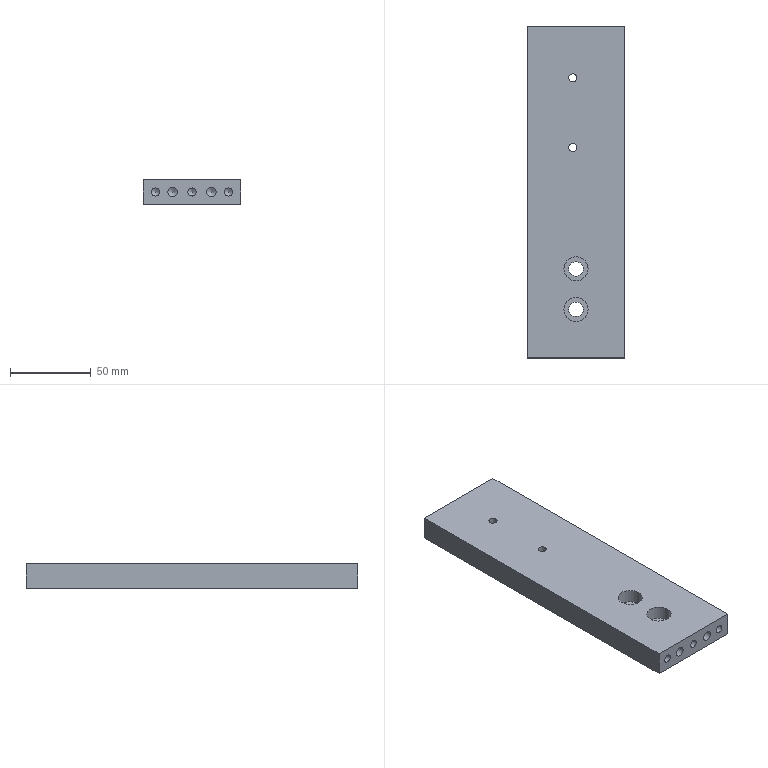Part | NX | features BREP 1 | 1 solid | 28 faces | box 60 x 205 x 15 mm | volume 177777 mm3 | cylinder 13 | plane 10 | cone 5 | commonest cylinder face diameters 5 x5 6 x2 9 x2 12 x2 15 x2
STEP:
#1=CARTESIAN_POINT('',(-4.5,27.5,7.5));
#2=VERTEX_POINT('',#1);
#3=CARTESIAN_POINT('',(-2.,27.5,7.5));
#4=DIRECTION('',(0.,0.,-1.));
#5=DIRECTION('',(-1.,0.,0.));
#6=AXIS2_PLACEMENT_3D('',#3,#4,#5);
#7=CIRCLE('',#6,2.5);
#8=EDGE_CURVE('',#2,#2,#7,.T.);
#9=ORIENTED_EDGE('',*,*,#8,.F.);
#10=EDGE_LOOP('',(#9));
#11=FACE_BOUND('',#10,.T.);
#12=CARTESIAN_POINT('',(-4.5,27.5,-4.));
#13=VERTEX_POINT('',#12);
#14=CARTESIAN_POINT('',(-2.,27.5,-4.));
#15=DIRECTION('',(0.,0.,1.));
#16=DIRECTION('',(-1.,0.,0.));
#17=AXIS2_PLACEMENT_3D('',#14,#15,#16);
#18=CIRCLE('',#17,2.5);
#19=EDGE_CURVE('',#13,#13,#18,.T.);
#20=ORIENTED_EDGE('',*,*,#19,.F.);
#21=EDGE_LOOP('',(#20));
#22=FACE_BOUND('',#21,.T.);
#23=CARTESIAN_POINT('',(-2.,27.5,-7.5));
#24=DIRECTION('',(0.,0.,-1.));
#25=DIRECTION('',(1.,0.,0.));
#26=AXIS2_PLACEMENT_3D('',#23,#24,#25);
#27=CYLINDRICAL_SURFACE('',#26,2.5);
#28=ADVANCED_FACE('',(#11,#22),#27,.F.);
#29=CARTESIAN_POINT('',(-4.5,70.5,7.5));
#30=VERTEX_POINT('',#29);
#31=CARTESIAN_POINT('',(-2.,70.5,7.5));
#32=DIRECTION('',(0.,0.,-1.));
#33=DIRECTION('',(-1.,0.,0.));
#34=AXIS2_PLACEMENT_3D('',#31,#32,#33);
#35=CIRCLE('',#34,2.5);
#36=EDGE_CURVE('',#30,#30,#35,.T.);
#37=ORIENTED_EDGE('',*,*,#36,.F.);
#38=EDGE_LOOP('',(#37));
#39=FACE_BOUND('',#38,.T.);
#40=CARTESIAN_POINT('',(-4.5,70.5,-4.));
#41=VERTEX_POINT('',#40);
#42=CARTESIAN_POINT('',(-2.,70.5,-4.));
#43=DIRECTION('',(0.,0.,1.));
#44=DIRECTION('',(-1.,0.,0.));
#45=AXIS2_PLACEMENT_3D('',#42,#43,#44);
#46=CIRCLE('',#45,2.5);
#47=EDGE_CURVE('',#41,#41,#46,.T.);
#48=ORIENTED_EDGE('',*,*,#47,.F.);
#49=EDGE_LOOP('',(#48));
#50=FACE_BOUND('',#49,.T.);
#51=CARTESIAN_POINT('',(-2.,70.5,-7.5));
#52=DIRECTION('',(0.,0.,-1.));
#53=DIRECTION('',(1.,0.,0.));
#54=AXIS2_PLACEMENT_3D('',#51,#52,#53);
#55=CYLINDRICAL_SURFACE('',#54,2.5);
#56=ADVANCED_FACE('',(#39,#50),#55,.F.);
#57=CARTESIAN_POINT('',(30.,-102.5,-7.5));
#58=VERTEX_POINT('',#57);
#59=CARTESIAN_POINT('',(30.,102.5,-7.5));
#60=VERTEX_POINT('',#59);
#61=CARTESIAN_POINT('',(30.,-102.5,-7.5));
#62=DIRECTION('',(0.,1.,0.));
#63=VECTOR('',#62,1000.);
#64=LINE('',#61,#63);
#65=EDGE_CURVE('',#58,#60,#64,.T.);
#66=ORIENTED_EDGE('',*,*,#65,.T.);
#67=CARTESIAN_POINT('',(30.,102.5,7.5));
#68=VERTEX_POINT('',#67);
#69=CARTESIAN_POINT('',(30.,102.5,7.5));
#70=DIRECTION('',(0.,0.,-1.));
#71=VECTOR('',#70,1000.);
#72=LINE('',#69,#71);
#73=EDGE_CURVE('',#68,#60,#72,.T.);
#74=ORIENTED_EDGE('',*,*,#73,.F.);
#75=CARTESIAN_POINT('',(30.,-102.5,7.5));
#76=VERTEX_POINT('',#75);
#77=CARTESIAN_POINT('',(30.,-102.5,7.5));
#78=DIRECTION('',(0.,1.,0.));
#79=VECTOR('',#78,1000.);
#80=LINE('',#77,#79);
#81=EDGE_CURVE('',#76,#68,#80,.T.);
#82=ORIENTED_EDGE('',*,*,#81,.F.);
#83=CARTESIAN_POINT('',(30.,-102.5,7.5));
#84=DIRECTION('',(0.,0.,-1.));
#85=VECTOR('',#84,1000.);
#86=LINE('',#83,#85);
#87=EDGE_CURVE('',#76,#58,#86,.T.);
#88=ORIENTED_EDGE('',*,*,#87,.T.);
#89=EDGE_LOOP('',(#66,#74,#82,#88));
#90=FACE_BOUND('',#89,.T.);
#91=CARTESIAN_POINT('',(30.,-102.5,7.5));
#92=DIRECTION('',(-1.,0.,0.));
#93=DIRECTION('',(0.,0.,-1.));
#94=AXIS2_PLACEMENT_3D('',#91,#92,#93);
#95=PLANE('',#94);
#96=ADVANCED_FACE('',(#90),#95,.F.);
#97=CARTESIAN_POINT('',(-30.,102.5,-7.5));
#98=VERTEX_POINT('',#97);
#99=CARTESIAN_POINT('',(-30.,102.5,-7.5));
#100=DIRECTION('',(-1.,0.,0.));
#101=VECTOR('',#100,1000.);
#102=LINE('',#99,#101);
#103=EDGE_CURVE('',#60,#98,#102,.T.);
#104=ORIENTED_EDGE('',*,*,#103,.T.);
#105=CARTESIAN_POINT('',(-30.,102.5,7.5));
#106=VERTEX_POINT('',#105);
#107=CARTESIAN_POINT('',(-30.,102.5,7.5));
#108=DIRECTION('',(0.,0.,-1.));
#109=VECTOR('',#108,1000.);
#110=LINE('',#107,#109);
#111=EDGE_CURVE('',#106,#98,#110,.T.);
#112=ORIENTED_EDGE('',*,*,#111,.F.);
#113=CARTESIAN_POINT('',(-30.,102.5,7.5));
#114=DIRECTION('',(-1.,0.,0.));
#115=VECTOR('',#114,1000.);
#116=LINE('',#113,#115);
#117=EDGE_CURVE('',#68,#106,#116,.T.);
#118=ORIENTED_EDGE('',*,*,#117,.F.);
#119=ORIENTED_EDGE('',*,*,#73,.T.);
#120=EDGE_LOOP('',(#104,#112,#118,#119));
#121=FACE_BOUND('',#120,.T.);
#122=CARTESIAN_POINT('',(-30.,102.5,7.5));
#123=DIRECTION('',(0.,-1.,0.));
#124=DIRECTION('',(0.,0.,1.));
#125=AXIS2_PLACEMENT_3D('',#122,#123,#124);
#126=PLANE('',#125);
#127=ADVANCED_FACE('',(#121),#126,.F.);
#128=CARTESIAN_POINT('',(-30.,-102.5,-7.5));
#129=VERTEX_POINT('',#128);
#130=CARTESIAN_POINT('',(-30.,-102.5,-7.5));
#131=DIRECTION('',(0.,-1.,0.));
#132=VECTOR('',#131,1000.);
#133=LINE('',#130,#132);
#134=EDGE_CURVE('',#98,#129,#133,.T.);
#135=ORIENTED_EDGE('',*,*,#134,.T.);
#136=CARTESIAN_POINT('',(-30.,-102.5,7.5));
#137=VERTEX_POINT('',#136);
#138=CARTESIAN_POINT('',(-30.,-102.5,7.5));
#139=DIRECTION('',(0.,0.,-1.));
#140=VECTOR('',#139,1000.);
#141=LINE('',#138,#140);
#142=EDGE_CURVE('',#137,#129,#141,.T.);
#143=ORIENTED_EDGE('',*,*,#142,.F.);
#144=CARTESIAN_POINT('',(-30.,-102.5,7.5));
#145=DIRECTION('',(0.,-1.,0.));
#146=VECTOR('',#145,1000.);
#147=LINE('',#144,#146);
#148=EDGE_CURVE('',#106,#137,#147,.T.);
#149=ORIENTED_EDGE('',*,*,#148,.F.);
#150=ORIENTED_EDGE('',*,*,#111,.T.);
#151=EDGE_LOOP('',(#135,#143,#149,#150));
#152=FACE_BOUND('',#151,.T.);
#153=CARTESIAN_POINT('',(-30.,-102.5,7.5));
#154=DIRECTION('',(1.,0.,0.));
#155=DIRECTION('',(0.,0.,1.));
#156=AXIS2_PLACEMENT_3D('',#153,#154,#155);
#157=PLANE('',#156);
#158=ADVANCED_FACE('',(#152),#157,.F.);
#159=CARTESIAN_POINT('',(-22.5,-102.5,-2.5));
#160=VERTEX_POINT('',#159);
#161=CARTESIAN_POINT('',(-22.5,-102.5,0.));
#162=DIRECTION('',(0.,-1.,0.));
#163=DIRECTION('',(0.,0.,-1.));
#164=AXIS2_PLACEMENT_3D('',#161,#162,#163);
#165=CIRCLE('',#164,2.5);
#166=EDGE_CURVE('',#160,#160,#165,.T.);
#167=ORIENTED_EDGE('',*,*,#166,.F.);
#168=EDGE_LOOP('',(#167));
#169=FACE_BOUND('',#168,.T.);
#170=CARTESIAN_POINT('',(0.,-102.5,-2.5));
#171=VERTEX_POINT('',#170);
#172=CARTESIAN_POINT('',(0.,-102.5,0.));
#173=DIRECTION('',(0.,-1.,0.));
#174=DIRECTION('',(0.,0.,-1.));
#175=AXIS2_PLACEMENT_3D('',#172,#173,#174);
#176=CIRCLE('',#175,2.5);
#177=EDGE_CURVE('',#171,#171,#176,.T.);
#178=ORIENTED_EDGE('',*,*,#177,.F.);
#179=EDGE_LOOP('',(#178));
#180=FACE_BOUND('',#179,.T.);
#181=CARTESIAN_POINT('',(22.5,-102.5,-2.5));
#182=VERTEX_POINT('',#181);
#183=CARTESIAN_POINT('',(22.5,-102.5,0.));
#184=DIRECTION('',(0.,-1.,0.));
#185=DIRECTION('',(0.,0.,-1.));
#186=AXIS2_PLACEMENT_3D('',#183,#184,#185);
#187=CIRCLE('',#186,2.5);
#188=EDGE_CURVE('',#182,#182,#187,.T.);
#189=ORIENTED_EDGE('',*,*,#188,.F.);
#190=EDGE_LOOP('',(#189));
#191=FACE_BOUND('',#190,.T.);
#192=CARTESIAN_POINT('',(12.,-102.5,-3.));
#193=VERTEX_POINT('',#192);
#194=CARTESIAN_POINT('',(12.,-102.5,0.));
#195=DIRECTION('',(0.,-1.,0.));
#196=DIRECTION('',(0.,0.,-1.));
#197=AXIS2_PLACEMENT_3D('',#194,#195,#196);
#198=CIRCLE('',#197,3.);
#199=EDGE_CURVE('',#193,#193,#198,.T.);
#200=ORIENTED_EDGE('',*,*,#199,.F.);
#201=EDGE_LOOP('',(#200));
#202=FACE_BOUND('',#201,.T.);
#203=CARTESIAN_POINT('',(-12.,-102.5,-3.));
#204=VERTEX_POINT('',#203);
#205=CARTESIAN_POINT('',(-12.,-102.5,0.));
#206=DIRECTION('',(0.,-1.,0.));
#207=DIRECTION('',(0.,0.,-1.));
#208=AXIS2_PLACEMENT_3D('',#205,#206,#207);
#209=CIRCLE('',#208,3.);
#210=EDGE_CURVE('',#204,#204,#209,.T.);
#211=ORIENTED_EDGE('',*,*,#210,.F.);
#212=EDGE_LOOP('',(#211));
#213=FACE_BOUND('',#212,.T.);
#214=CARTESIAN_POINT('',(-30.,-102.5,-7.5));
#215=DIRECTION('',(1.,0.,0.));
#216=VECTOR('',#215,1000.);
#217=LINE('',#214,#216);
#218=EDGE_CURVE('',#129,#58,#217,.T.);
#219=ORIENTED_EDGE('',*,*,#218,.T.);
#220=ORIENTED_EDGE('',*,*,#87,.F.);
#221=CARTESIAN_POINT('',(-30.,-102.5,7.5));
#222=DIRECTION('',(1.,0.,0.));
#223=VECTOR('',#222,1000.);
#224=LINE('',#221,#223);
#225=EDGE_CURVE('',#137,#76,#224,.T.);
#226=ORIENTED_EDGE('',*,*,#225,.F.);
#227=ORIENTED_EDGE('',*,*,#142,.T.);
#228=EDGE_LOOP('',(#219,#220,#226,#227));
#229=FACE_BOUND('',#228,.T.);
#230=CARTESIAN_POINT('',(-30.,-102.5,7.5));
#231=DIRECTION('',(0.,1.,0.));
#232=DIRECTION('',(0.,0.,-1.));
#233=AXIS2_PLACEMENT_3D('',#230,#231,#232);
#234=PLANE('',#233);
#235=ADVANCED_FACE('',(#169,#180,#191,#202,#213,#229),#234,.F.);
#236=CARTESIAN_POINT('',(7.5,-72.5,7.5));
#237=VERTEX_POINT('',#236);
#238=CARTESIAN_POINT('',(0.,-72.5,7.5));
#239=DIRECTION('',(0.,0.,1.));
#240=DIRECTION('',(1.,0.,0.));
#241=AXIS2_PLACEMENT_3D('',#238,#239,#240);
#242=CIRCLE('',#241,7.5);
#243=EDGE_CURVE('',#237,#237,#242,.T.);
#244=ORIENTED_EDGE('',*,*,#243,.F.);
#245=EDGE_LOOP('',(#244));
#246=FACE_BOUND('',#245,.T.);
#247=CARTESIAN_POINT('',(7.5,-47.5,7.5));
#248=VERTEX_POINT('',#247);
#249=CARTESIAN_POINT('',(0.,-47.5,7.5));
#250=DIRECTION('',(0.,0.,1.));
#251=DIRECTION('',(1.,0.,0.));
#252=AXIS2_PLACEMENT_3D('',#249,#250,#251);
#253=CIRCLE('',#252,7.5);
#254=EDGE_CURVE('',#248,#248,#253,.T.);
#255=ORIENTED_EDGE('',*,*,#254,.F.);
#256=EDGE_LOOP('',(#255));
#257=FACE_BOUND('',#256,.T.);
#258=ORIENTED_EDGE('',*,*,#36,.T.);
#259=EDGE_LOOP('',(#258));
#260=FACE_BOUND('',#259,.T.);
#261=ORIENTED_EDGE('',*,*,#8,.T.);
#262=EDGE_LOOP('',(#261));
#263=FACE_BOUND('',#262,.T.);
#264=ORIENTED_EDGE('',*,*,#81,.T.);
#265=ORIENTED_EDGE('',*,*,#117,.T.);
#266=ORIENTED_EDGE('',*,*,#148,.T.);
#267=ORIENTED_EDGE('',*,*,#225,.T.);
#268=EDGE_LOOP('',(#264,#265,#266,#267));
#269=FACE_BOUND('',#268,.T.);
#270=CARTESIAN_POINT('',(0.,0.,7.5));
#271=DIRECTION('',(0.,0.,-1.));
#272=DIRECTION('',(1.,0.,0.));
#273=AXIS2_PLACEMENT_3D('',#270,#271,#272);
#274=PLANE('',#273);
#275=ADVANCED_FACE('',(#246,#257,#260,#263,#269),#274,.F.);
#276=CARTESIAN_POINT('',(4.5,-72.5,-7.5));
#277=VERTEX_POINT('',#276);
#278=CARTESIAN_POINT('',(0.,-72.5,-7.5));
#279=DIRECTION('',(0.,0.,1.));
#280=DIRECTION('',(1.,0.,0.));
#281=AXIS2_PLACEMENT_3D('',#278,#279,#280);
#282=CIRCLE('',#281,4.5);
#283=EDGE_CURVE('',#277,#277,#282,.T.);
#284=ORIENTED_EDGE('',*,*,#283,.T.);
#285=EDGE_LOOP('',(#284));
#286=FACE_BOUND('',#285,.T.);
#287=CARTESIAN_POINT('',(4.5,-47.5,-7.5));
#288=VERTEX_POINT('',#287);
#289=CARTESIAN_POINT('',(0.,-47.5,-7.5));
#290=DIRECTION('',(0.,0.,1.));
#291=DIRECTION('',(1.,0.,0.));
#292=AXIS2_PLACEMENT_3D('',#289,#290,#291);
#293=CIRCLE('',#292,4.5);
#294=EDGE_CURVE('',#288,#288,#293,.T.);
#295=ORIENTED_EDGE('',*,*,#294,.T.);
#296=EDGE_LOOP('',(#295));
#297=FACE_BOUND('',#296,.T.);
#298=CARTESIAN_POINT('',(-8.,70.5,-7.5));
#299=VERTEX_POINT('',#298);
#300=CARTESIAN_POINT('',(-2.,70.5,-7.5));
#301=DIRECTION('',(0.,0.,-1.));
#302=DIRECTION('',(-1.,0.,0.));
#303=AXIS2_PLACEMENT_3D('',#300,#301,#302);
#304=CIRCLE('',#303,6.);
#305=EDGE_CURVE('',#299,#299,#304,.T.);
#306=ORIENTED_EDGE('',*,*,#305,.F.);
#307=EDGE_LOOP('',(#306));
#308=FACE_BOUND('',#307,.T.);
#309=CARTESIAN_POINT('',(-8.,27.5,-7.5));
#310=VERTEX_POINT('',#309);
#311=CARTESIAN_POINT('',(-2.,27.5,-7.5));
#312=DIRECTION('',(0.,0.,-1.));
#313=DIRECTION('',(-1.,0.,0.));
#314=AXIS2_PLACEMENT_3D('',#311,#312,#313);
#315=CIRCLE('',#314,6.);
#316=EDGE_CURVE('',#310,#310,#315,.T.);
#317=ORIENTED_EDGE('',*,*,#316,.F.);
#318=EDGE_LOOP('',(#317));
#319=FACE_BOUND('',#318,.T.);
#320=ORIENTED_EDGE('',*,*,#65,.F.);
#321=ORIENTED_EDGE('',*,*,#218,.F.);
#322=ORIENTED_EDGE('',*,*,#134,.F.);
#323=ORIENTED_EDGE('',*,*,#103,.F.);
#324=EDGE_LOOP('',(#320,#321,#322,#323));
#325=FACE_BOUND('',#324,.T.);
#326=CARTESIAN_POINT('',(0.,0.,-7.5));
#327=DIRECTION('',(0.,0.,-1.));
#328=DIRECTION('',(1.,0.,0.));
#329=AXIS2_PLACEMENT_3D('',#326,#327,#328);
#330=PLANE('',#329);
#331=ADVANCED_FACE('',(#286,#297,#308,#319,#325),#330,.T.);
#332=CARTESIAN_POINT('',(-8.,70.5,-4.));
#333=VERTEX_POINT('',#332);
#334=CARTESIAN_POINT('',(-2.,70.5,-4.));
#335=DIRECTION('',(0.,0.,-1.));
#336=DIRECTION('',(-1.,0.,0.));
#337=AXIS2_PLACEMENT_3D('',#334,#335,#336);
#338=CIRCLE('',#337,6.);
#339=EDGE_CURVE('',#333,#333,#338,.T.);
#340=ORIENTED_EDGE('',*,*,#339,.T.);
#341=EDGE_LOOP('',(#340));
#342=FACE_BOUND('',#341,.T.);
#343=ORIENTED_EDGE('',*,*,#47,.T.);
#344=EDGE_LOOP('',(#343));
#345=FACE_BOUND('',#344,.T.);
#346=CARTESIAN_POINT('',(-2.,70.5,-4.));
#347=DIRECTION('',(0.,0.,-1.));
#348=DIRECTION('',(1.,0.,0.));
#349=AXIS2_PLACEMENT_3D('',#346,#347,#348);
#350=PLANE('',#349);
#351=ADVANCED_FACE('',(#342,#345),#350,.T.);
#352=ORIENTED_EDGE('',*,*,#339,.F.);
#353=EDGE_LOOP('',(#352));
#354=FACE_BOUND('',#353,.T.);
#355=ORIENTED_EDGE('',*,*,#305,.T.);
#356=EDGE_LOOP('',(#355));
#357=FACE_BOUND('',#356,.T.);
#358=CARTESIAN_POINT('',(-2.,70.5,-4.));
#359=DIRECTION('',(0.,0.,-1.));
#360=DIRECTION('',(1.,0.,0.));
#361=AXIS2_PLACEMENT_3D('',#358,#359,#360);
#362=CYLINDRICAL_SURFACE('',#361,6.);
#363=ADVANCED_FACE('',(#354,#357),#362,.F.);
#364=CARTESIAN_POINT('',(-8.,27.5,-4.));
#365=VERTEX_POINT('',#364);
#366=CARTESIAN_POINT('',(-2.,27.5,-4.));
#367=DIRECTION('',(0.,0.,-1.));
#368=DIRECTION('',(-1.,0.,0.));
#369=AXIS2_PLACEMENT_3D('',#366,#367,#368);
#370=CIRCLE('',#369,6.);
#371=EDGE_CURVE('',#365,#365,#370,.T.);
#372=ORIENTED_EDGE('',*,*,#371,.T.);
#373=EDGE_LOOP('',(#372));
#374=FACE_BOUND('',#373,.T.);
#375=ORIENTED_EDGE('',*,*,#19,.T.);
#376=EDGE_LOOP('',(#375));
#377=FACE_BOUND('',#376,.T.);
#378=CARTESIAN_POINT('',(-2.,27.5,-4.));
#379=DIRECTION('',(0.,0.,-1.));
#380=DIRECTION('',(1.,0.,0.));
#381=AXIS2_PLACEMENT_3D('',#378,#379,#380);
#382=PLANE('',#381);
#383=ADVANCED_FACE('',(#374,#377),#382,.T.);
#384=ORIENTED_EDGE('',*,*,#371,.F.);
#385=EDGE_LOOP('',(#384));
#386=FACE_BOUND('',#385,.T.);
#387=ORIENTED_EDGE('',*,*,#316,.T.);
#388=EDGE_LOOP('',(#387));
#389=FACE_BOUND('',#388,.T.);
#390=CARTESIAN_POINT('',(-2.,27.5,-4.));
#391=DIRECTION('',(0.,0.,-1.));
#392=DIRECTION('',(1.,0.,0.));
#393=AXIS2_PLACEMENT_3D('',#390,#391,#392);
#394=CYLINDRICAL_SURFACE('',#393,6.);
#395=ADVANCED_FACE('',(#386,#389),#394,.F.);
#396=CARTESIAN_POINT('',(-12.,-88.697,0.));
#397=VERTEX_POINT('',#396);
#398=VERTEX_LOOP('',#397);
#399=FACE_BOUND('',#398,.T.);
#400=CARTESIAN_POINT('',(-12.,-90.5,-3.));
#401=VERTEX_POINT('',#400);
#402=CARTESIAN_POINT('',(-12.,-90.5,0.));
#403=DIRECTION('',(0.,-1.,0.));
#404=DIRECTION('',(0.,0.,-1.));
#405=AXIS2_PLACEMENT_3D('',#402,#403,#404);
#406=CIRCLE('',#405,3.);
#407=EDGE_CURVE('',#401,#401,#406,.T.);
#408=ORIENTED_EDGE('',*,*,#407,.T.);
#409=EDGE_LOOP('',(#408));
#410=FACE_BOUND('',#409,.T.);
#411=CARTESIAN_POINT('',(-12.,-90.5,0.));
#412=DIRECTION('',(0.,-1.,0.));
#413=DIRECTION('',(0.,0.,1.));
#414=AXIS2_PLACEMENT_3D('',#411,#412,#413);
#415=CONICAL_SURFACE('',#414,3.,1.03);
#416=ADVANCED_FACE('',(#399,#410),#415,.F.);
#417=ORIENTED_EDGE('',*,*,#407,.F.);
#418=EDGE_LOOP('',(#417));
#419=FACE_BOUND('',#418,.T.);
#420=ORIENTED_EDGE('',*,*,#210,.T.);
#421=EDGE_LOOP('',(#420));
#422=FACE_BOUND('',#421,.T.);
#423=CARTESIAN_POINT('',(-12.,-102.5,0.));
#424=DIRECTION('',(0.,-1.,0.));
#425=DIRECTION('',(0.,0.,1.));
#426=AXIS2_PLACEMENT_3D('',#423,#424,#425);
#427=CYLINDRICAL_SURFACE('',#426,3.);
#428=ADVANCED_FACE('',(#419,#422),#427,.F.);
#429=CARTESIAN_POINT('',(12.,-88.697,0.));
#430=VERTEX_POINT('',#429);
#431=VERTEX_LOOP('',#430);
#432=FACE_BOUND('',#431,.T.);
#433=CARTESIAN_POINT('',(12.,-90.5,-3.));
#434=VERTEX_POINT('',#433);
#435=CARTESIAN_POINT('',(12.,-90.5,0.));
#436=DIRECTION('',(0.,-1.,0.));
#437=DIRECTION('',(0.,0.,-1.));
#438=AXIS2_PLACEMENT_3D('',#435,#436,#437);
#439=CIRCLE('',#438,3.);
#440=EDGE_CURVE('',#434,#434,#439,.T.);
#441=ORIENTED_EDGE('',*,*,#440,.T.);
#442=EDGE_LOOP('',(#441));
#443=FACE_BOUND('',#442,.T.);
#444=CARTESIAN_POINT('',(12.,-90.5,0.));
#445=DIRECTION('',(0.,-1.,0.));
#446=DIRECTION('',(0.,0.,1.));
#447=AXIS2_PLACEMENT_3D('',#444,#445,#446);
#448=CONICAL_SURFACE('',#447,3.,1.03);
#449=ADVANCED_FACE('',(#432,#443),#448,.F.);
#450=ORIENTED_EDGE('',*,*,#440,.F.);
#451=EDGE_LOOP('',(#450));
#452=FACE_BOUND('',#451,.T.);
#453=ORIENTED_EDGE('',*,*,#199,.T.);
#454=EDGE_LOOP('',(#453));
#455=FACE_BOUND('',#454,.T.);
#456=CARTESIAN_POINT('',(12.,-102.5,0.));
#457=DIRECTION('',(0.,-1.,0.));
#458=DIRECTION('',(0.,0.,1.));
#459=AXIS2_PLACEMENT_3D('',#456,#457,#458);
#460=CYLINDRICAL_SURFACE('',#459,3.);
#461=ADVANCED_FACE('',(#452,#455),#460,.F.);
#462=CARTESIAN_POINT('',(22.5,-85.998,0.));
#463=VERTEX_POINT('',#462);
#464=VERTEX_LOOP('',#463);
#465=FACE_BOUND('',#464,.T.);
#466=CARTESIAN_POINT('',(22.5,-87.5,-2.5));
#467=VERTEX_POINT('',#466);
#468=CARTESIAN_POINT('',(22.5,-87.5,0.));
#469=DIRECTION('',(0.,-1.,0.));
#470=DIRECTION('',(0.,0.,-1.));
#471=AXIS2_PLACEMENT_3D('',#468,#469,#470);
#472=CIRCLE('',#471,2.5);
#473=EDGE_CURVE('',#467,#467,#472,.T.);
#474=ORIENTED_EDGE('',*,*,#473,.T.);
#475=EDGE_LOOP('',(#474));
#476=FACE_BOUND('',#475,.T.);
#477=CARTESIAN_POINT('',(22.5,-87.5,0.));
#478=DIRECTION('',(0.,-1.,0.));
#479=DIRECTION('',(0.,0.,1.));
#480=AXIS2_PLACEMENT_3D('',#477,#478,#479);
#481=CONICAL_SURFACE('',#480,2.5,1.03);
#482=ADVANCED_FACE('',(#465,#476),#481,.F.);
#483=ORIENTED_EDGE('',*,*,#473,.F.);
#484=EDGE_LOOP('',(#483));
#485=FACE_BOUND('',#484,.T.);
#486=ORIENTED_EDGE('',*,*,#188,.T.);
#487=EDGE_LOOP('',(#486));
#488=FACE_BOUND('',#487,.T.);
#489=CARTESIAN_POINT('',(22.5,-102.5,0.));
#490=DIRECTION('',(0.,-1.,0.));
#491=DIRECTION('',(0.,0.,1.));
#492=AXIS2_PLACEMENT_3D('',#489,#490,#491);
#493=CYLINDRICAL_SURFACE('',#492,2.5);
#494=ADVANCED_FACE('',(#485,#488),#493,.F.);
#495=CARTESIAN_POINT('',(0.,-85.998,0.));
#496=VERTEX_POINT('',#495);
#497=VERTEX_LOOP('',#496);
#498=FACE_BOUND('',#497,.T.);
#499=CARTESIAN_POINT('',(0.,-87.5,-2.5));
#500=VERTEX_POINT('',#499);
#501=CARTESIAN_POINT('',(0.,-87.5,0.));
#502=DIRECTION('',(0.,-1.,0.));
#503=DIRECTION('',(0.,0.,-1.));
#504=AXIS2_PLACEMENT_3D('',#501,#502,#503);
#505=CIRCLE('',#504,2.5);
#506=EDGE_CURVE('',#500,#500,#505,.T.);
#507=ORIENTED_EDGE('',*,*,#506,.T.);
#508=EDGE_LOOP('',(#507));
#509=FACE_BOUND('',#508,.T.);
#510=CARTESIAN_POINT('',(0.,-87.5,0.));
#511=DIRECTION('',(0.,-1.,0.));
#512=DIRECTION('',(0.,0.,1.));
#513=AXIS2_PLACEMENT_3D('',#510,#511,#512);
#514=CONICAL_SURFACE('',#513,2.5,1.03);
#515=ADVANCED_FACE('',(#498,#509),#514,.F.);
#516=ORIENTED_EDGE('',*,*,#506,.F.);
#517=EDGE_LOOP('',(#516));
#518=FACE_BOUND('',#517,.T.);
#519=ORIENTED_EDGE('',*,*,#177,.T.);
#520=EDGE_LOOP('',(#519));
#521=FACE_BOUND('',#520,.T.);
#522=CARTESIAN_POINT('',(0.,-102.5,0.));
#523=DIRECTION('',(0.,-1.,0.));
#524=DIRECTION('',(0.,0.,1.));
#525=AXIS2_PLACEMENT_3D('',#522,#523,#524);
#526=CYLINDRICAL_SURFACE('',#525,2.5);
#527=ADVANCED_FACE('',(#518,#521),#526,.F.);
#528=CARTESIAN_POINT('',(-22.5,-85.998,0.));
#529=VERTEX_POINT('',#528);
#530=VERTEX_LOOP('',#529);
#531=FACE_BOUND('',#530,.T.);
#532=CARTESIAN_POINT('',(-22.5,-87.5,-2.5));
#533=VERTEX_POINT('',#532);
#534=CARTESIAN_POINT('',(-22.5,-87.5,0.));
#535=DIRECTION('',(0.,-1.,0.));
#536=DIRECTION('',(0.,0.,-1.));
#537=AXIS2_PLACEMENT_3D('',#534,#535,#536);
#538=CIRCLE('',#537,2.5);
#539=EDGE_CURVE('',#533,#533,#538,.T.);
#540=ORIENTED_EDGE('',*,*,#539,.T.);
#541=EDGE_LOOP('',(#540));
#542=FACE_BOUND('',#541,.T.);
#543=CARTESIAN_POINT('',(-22.5,-87.5,0.));
#544=DIRECTION('',(0.,-1.,0.));
#545=DIRECTION('',(0.,0.,1.));
#546=AXIS2_PLACEMENT_3D('',#543,#544,#545);
#547=CONICAL_SURFACE('',#546,2.5,1.03);
#548=ADVANCED_FACE('',(#531,#542),#547,.F.);
#549=ORIENTED_EDGE('',*,*,#539,.F.);
#550=EDGE_LOOP('',(#549));
#551=FACE_BOUND('',#550,.T.);
#552=ORIENTED_EDGE('',*,*,#166,.T.);
#553=EDGE_LOOP('',(#552));
#554=FACE_BOUND('',#553,.T.);
#555=CARTESIAN_POINT('',(-22.5,-102.5,0.));
#556=DIRECTION('',(0.,-1.,0.));
#557=DIRECTION('',(0.,0.,1.));
#558=AXIS2_PLACEMENT_3D('',#555,#556,#557);
#559=CYLINDRICAL_SURFACE('',#558,2.5);
#560=ADVANCED_FACE('',(#551,#554),#559,.F.);
#561=ORIENTED_EDGE('',*,*,#294,.F.);
#562=EDGE_LOOP('',(#561));
#563=FACE_BOUND('',#562,.T.);
#564=CARTESIAN_POINT('',(4.5,-47.5,-1.1));
#565=VERTEX_POINT('',#564);
#566=CARTESIAN_POINT('',(0.,-47.5,-1.1));
#567=DIRECTION('',(0.,0.,1.));
#568=DIRECTION('',(1.,0.,0.));
#569=AXIS2_PLACEMENT_3D('',#566,#567,#568);
#570=CIRCLE('',#569,4.5);
#571=EDGE_CURVE('',#565,#565,#570,.T.);
#572=ORIENTED_EDGE('',*,*,#571,.T.);
#573=EDGE_LOOP('',(#572));
#574=FACE_BOUND('',#573,.T.);
#575=CARTESIAN_POINT('',(0.,-47.5,7.5));
#576=DIRECTION('',(0.,0.,1.));
#577=DIRECTION('',(-1.,0.,0.));
#578=AXIS2_PLACEMENT_3D('',#575,#576,#577);
#579=CYLINDRICAL_SURFACE('',#578,4.5);
#580=ADVANCED_FACE('',(#563,#574),#579,.F.);
#581=ORIENTED_EDGE('',*,*,#571,.F.);
#582=EDGE_LOOP('',(#581));
#583=FACE_BOUND('',#582,.T.);
#584=CARTESIAN_POINT('',(7.5,-47.5,-1.1));
#585=VERTEX_POINT('',#584);
#586=CARTESIAN_POINT('',(0.,-47.5,-1.1));
#587=DIRECTION('',(0.,0.,1.));
#588=DIRECTION('',(1.,0.,0.));
#589=AXIS2_PLACEMENT_3D('',#586,#587,#588);
#590=CIRCLE('',#589,7.5);
#591=EDGE_CURVE('',#585,#585,#590,.T.);
#592=ORIENTED_EDGE('',*,*,#591,.T.);
#593=EDGE_LOOP('',(#592));
#594=FACE_BOUND('',#593,.T.);
#595=CARTESIAN_POINT('',(4.5,-47.5,-1.1));
#596=DIRECTION('',(0.,0.,-1.));
#597=DIRECTION('',(1.,0.,0.));
#598=AXIS2_PLACEMENT_3D('',#595,#596,#597);
#599=PLANE('',#598);
#600=ADVANCED_FACE('',(#583,#594),#599,.F.);
#601=ORIENTED_EDGE('',*,*,#591,.F.);
#602=EDGE_LOOP('',(#601));
#603=FACE_BOUND('',#602,.T.);
#604=ORIENTED_EDGE('',*,*,#254,.T.);
#605=EDGE_LOOP('',(#604));
#606=FACE_BOUND('',#605,.T.);
#607=CARTESIAN_POINT('',(0.,-47.5,7.5));
#608=DIRECTION('',(0.,0.,1.));
#609=DIRECTION('',(-1.,0.,0.));
#610=AXIS2_PLACEMENT_3D('',#607,#608,#609);
#611=CYLINDRICAL_SURFACE('',#610,7.5);
#612=ADVANCED_FACE('',(#603,#606),#611,.F.);
#613=ORIENTED_EDGE('',*,*,#283,.F.);
#614=EDGE_LOOP('',(#613));
#615=FACE_BOUND('',#614,.T.);
#616=CARTESIAN_POINT('',(4.5,-72.5,-1.1));
#617=VERTEX_POINT('',#616);
#618=CARTESIAN_POINT('',(0.,-72.5,-1.1));
#619=DIRECTION('',(0.,0.,1.));
#620=DIRECTION('',(1.,0.,0.));
#621=AXIS2_PLACEMENT_3D('',#618,#619,#620);
#622=CIRCLE('',#621,4.5);
#623=EDGE_CURVE('',#617,#617,#622,.T.);
#624=ORIENTED_EDGE('',*,*,#623,.T.);
#625=EDGE_LOOP('',(#624));
#626=FACE_BOUND('',#625,.T.);
#627=CARTESIAN_POINT('',(0.,-72.5,7.5));
#628=DIRECTION('',(0.,0.,1.));
#629=DIRECTION('',(-1.,0.,0.));
#630=AXIS2_PLACEMENT_3D('',#627,#628,#629);
#631=CYLINDRICAL_SURFACE('',#630,4.5);
#632=ADVANCED_FACE('',(#615,#626),#631,.F.);
#633=ORIENTED_EDGE('',*,*,#623,.F.);
#634=EDGE_LOOP('',(#633));
#635=FACE_BOUND('',#634,.T.);
#636=CARTESIAN_POINT('',(7.5,-72.5,-1.1));
#637=VERTEX_POINT('',#636);
#638=CARTESIAN_POINT('',(0.,-72.5,-1.1));
#639=DIRECTION('',(0.,0.,1.));
#640=DIRECTION('',(1.,0.,0.));
#641=AXIS2_PLACEMENT_3D('',#638,#639,#640);
#642=CIRCLE('',#641,7.5);
#643=EDGE_CURVE('',#637,#637,#642,.T.);
#644=ORIENTED_EDGE('',*,*,#643,.T.);
#645=EDGE_LOOP('',(#644));
#646=FACE_BOUND('',#645,.T.);
#647=CARTESIAN_POINT('',(4.5,-72.5,-1.1));
#648=DIRECTION('',(0.,0.,-1.));
#649=DIRECTION('',(1.,0.,0.));
#650=AXIS2_PLACEMENT_3D('',#647,#648,#649);
#651=PLANE('',#650);
#652=ADVANCED_FACE('',(#635,#646),#651,.F.);
#653=ORIENTED_EDGE('',*,*,#643,.F.);
#654=EDGE_LOOP('',(#653));
#655=FACE_BOUND('',#654,.T.);
#656=ORIENTED_EDGE('',*,*,#243,.T.);
#657=EDGE_LOOP('',(#656));
#658=FACE_BOUND('',#657,.T.);
#659=CARTESIAN_POINT('',(0.,-72.5,7.5));
#660=DIRECTION('',(0.,0.,1.));
#661=DIRECTION('',(-1.,0.,0.));
#662=AXIS2_PLACEMENT_3D('',#659,#660,#661);
#663=CYLINDRICAL_SURFACE('',#662,7.5);
#664=ADVANCED_FACE('',(#655,#658),#663,.F.);
#665=CLOSED_SHELL('',(#28,#56,#96,#127,#158,#235,#275,#331,#351,#363,#383,#395,#416,#428,#449,#461,#482,#494,#515,#527,#548,#560,#580,#600,#612,#632,#652,#664));
#666=MANIFOLD_SOLID_BREP('',#665);
#667=(LENGTH_UNIT()NAMED_UNIT(*)SI_UNIT(.MILLI.,.METRE.));
#668=UNCERTAINTY_MEASURE_WITH_UNIT(LENGTH_MEASURE(0.00001),#667,'','');
#669=(NAMED_UNIT(*)PLANE_ANGLE_UNIT()SI_UNIT($,.RADIAN.));
#670=(NAMED_UNIT(*)SI_UNIT($,.STERADIAN.)SOLID_ANGLE_UNIT());
#671=(GEOMETRIC_REPRESENTATION_CONTEXT(3)GLOBAL_UNCERTAINTY_ASSIGNED_CONTEXT((#668))GLOBAL_UNIT_ASSIGNED_CONTEXT((#667,#669,#670))REPRESENTATION_CONTEXT('',''));
#672=ADVANCED_BREP_SHAPE_REPRESENTATION('',(#666),#671);